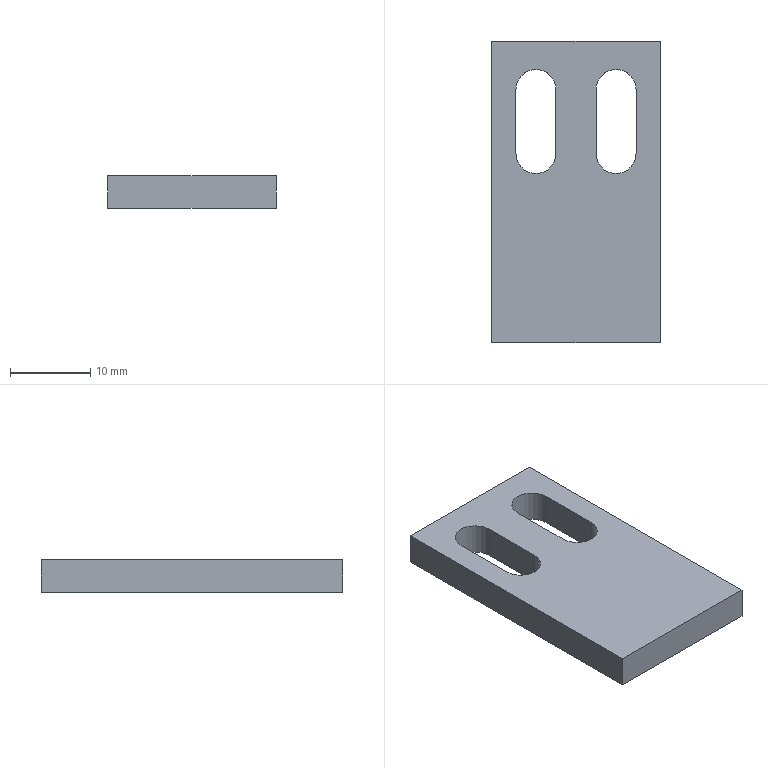Part | STEP file | Sensor spacer block | 1 solid | 14 faces | box 21 x 37.576 x 4 mm | volume 2679 mm3 | plane 10 | cylinder 4 | commonest cylinder face diameters 5 x4
STEP:
#1=CARTESIAN_POINT('',(-11.,-10.,0.));
#2=VERTEX_POINT('',#1);
#3=CARTESIAN_POINT('',(-11.,-47.576,0.));
#4=VERTEX_POINT('',#3);
#5=CARTESIAN_POINT('',(-11.,-10.,0.));
#6=DIRECTION('',(0.,-1.,0.));
#7=VECTOR('',#6,1000.);
#8=LINE('',#5,#7);
#9=EDGE_CURVE('',#2,#4,#8,.T.);
#10=ORIENTED_EDGE('',*,*,#9,.T.);
#11=CARTESIAN_POINT('',(-11.,-47.576,4.));
#12=VERTEX_POINT('',#11);
#13=CARTESIAN_POINT('',(-11.,-47.576,4.));
#14=DIRECTION('',(0.,0.,-1.));
#15=VECTOR('',#14,1000.);
#16=LINE('',#13,#15);
#17=EDGE_CURVE('',#12,#4,#16,.T.);
#18=ORIENTED_EDGE('',*,*,#17,.F.);
#19=CARTESIAN_POINT('',(-11.,-10.,4.));
#20=VERTEX_POINT('',#19);
#21=CARTESIAN_POINT('',(-11.,-10.,4.));
#22=DIRECTION('',(0.,-1.,0.));
#23=VECTOR('',#22,1000.);
#24=LINE('',#21,#23);
#25=EDGE_CURVE('',#20,#12,#24,.T.);
#26=ORIENTED_EDGE('',*,*,#25,.F.);
#27=CARTESIAN_POINT('',(-11.,-10.,4.));
#28=DIRECTION('',(0.,0.,-1.));
#29=VECTOR('',#28,1000.);
#30=LINE('',#27,#29);
#31=EDGE_CURVE('',#20,#2,#30,.T.);
#32=ORIENTED_EDGE('',*,*,#31,.T.);
#33=EDGE_LOOP('',(#10,#18,#26,#32));
#34=FACE_OUTER_BOUND('',#33,.T.);
#35=CARTESIAN_POINT('',(-11.,-10.,4.));
#36=DIRECTION('',(1.,0.,0.));
#37=DIRECTION('',(0.,0.,-1.));
#38=AXIS2_PLACEMENT_3D('',#35,#36,#37);
#39=PLANE('',#38);
#40=ADVANCED_FACE('',(#34),#39,.F.);
#41=CARTESIAN_POINT('',(10.,-47.576,0.));
#42=VERTEX_POINT('',#41);
#43=CARTESIAN_POINT('',(-11.,-47.576,0.));
#44=DIRECTION('',(1.,0.,0.));
#45=VECTOR('',#44,1000.);
#46=LINE('',#43,#45);
#47=EDGE_CURVE('',#4,#42,#46,.T.);
#48=ORIENTED_EDGE('',*,*,#47,.T.);
#49=CARTESIAN_POINT('',(10.,-47.576,4.));
#50=VERTEX_POINT('',#49);
#51=CARTESIAN_POINT('',(10.,-47.576,4.));
#52=DIRECTION('',(0.,0.,-1.));
#53=VECTOR('',#52,1000.);
#54=LINE('',#51,#53);
#55=EDGE_CURVE('',#50,#42,#54,.T.);
#56=ORIENTED_EDGE('',*,*,#55,.F.);
#57=CARTESIAN_POINT('',(-11.,-47.576,4.));
#58=DIRECTION('',(1.,0.,0.));
#59=VECTOR('',#58,1000.);
#60=LINE('',#57,#59);
#61=EDGE_CURVE('',#12,#50,#60,.T.);
#62=ORIENTED_EDGE('',*,*,#61,.F.);
#63=ORIENTED_EDGE('',*,*,#17,.T.);
#64=EDGE_LOOP('',(#48,#56,#62,#63));
#65=FACE_OUTER_BOUND('',#64,.T.);
#66=CARTESIAN_POINT('',(-11.,-47.576,4.));
#67=DIRECTION('',(0.,1.,0.));
#68=DIRECTION('',(0.,0.,1.));
#69=AXIS2_PLACEMENT_3D('',#66,#67,#68);
#70=PLANE('',#69);
#71=ADVANCED_FACE('',(#65),#70,.F.);
#72=CARTESIAN_POINT('',(10.,-10.,0.));
#73=VERTEX_POINT('',#72);
#74=CARTESIAN_POINT('',(10.,-10.,0.));
#75=DIRECTION('',(0.,1.,0.));
#76=VECTOR('',#75,1000.);
#77=LINE('',#74,#76);
#78=EDGE_CURVE('',#42,#73,#77,.T.);
#79=ORIENTED_EDGE('',*,*,#78,.T.);
#80=CARTESIAN_POINT('',(10.,-10.,4.));
#81=VERTEX_POINT('',#80);
#82=CARTESIAN_POINT('',(10.,-10.,4.));
#83=DIRECTION('',(0.,0.,-1.));
#84=VECTOR('',#83,1000.);
#85=LINE('',#82,#84);
#86=EDGE_CURVE('',#81,#73,#85,.T.);
#87=ORIENTED_EDGE('',*,*,#86,.F.);
#88=CARTESIAN_POINT('',(10.,-10.,4.));
#89=DIRECTION('',(0.,1.,0.));
#90=VECTOR('',#89,1000.);
#91=LINE('',#88,#90);
#92=EDGE_CURVE('',#50,#81,#91,.T.);
#93=ORIENTED_EDGE('',*,*,#92,.F.);
#94=ORIENTED_EDGE('',*,*,#55,.T.);
#95=EDGE_LOOP('',(#79,#87,#93,#94));
#96=FACE_OUTER_BOUND('',#95,.T.);
#97=CARTESIAN_POINT('',(10.,-10.,4.));
#98=DIRECTION('',(-1.,0.,0.));
#99=DIRECTION('',(0.,-1.,0.));
#100=AXIS2_PLACEMENT_3D('',#97,#98,#99);
#101=PLANE('',#100);
#102=ADVANCED_FACE('',(#96),#101,.F.);
#103=CARTESIAN_POINT('',(-11.,-10.,0.));
#104=DIRECTION('',(-1.,0.,0.));
#105=VECTOR('',#104,1000.);
#106=LINE('',#103,#105);
#107=EDGE_CURVE('',#73,#2,#106,.T.);
#108=ORIENTED_EDGE('',*,*,#107,.T.);
#109=ORIENTED_EDGE('',*,*,#31,.F.);
#110=CARTESIAN_POINT('',(-11.,-10.,4.));
#111=DIRECTION('',(-1.,0.,0.));
#112=VECTOR('',#111,1000.);
#113=LINE('',#110,#112);
#114=EDGE_CURVE('',#81,#20,#113,.T.);
#115=ORIENTED_EDGE('',*,*,#114,.F.);
#116=ORIENTED_EDGE('',*,*,#86,.T.);
#117=EDGE_LOOP('',(#108,#109,#115,#116));
#118=FACE_OUTER_BOUND('',#117,.T.);
#119=CARTESIAN_POINT('',(-11.,-10.,4.));
#120=DIRECTION('',(0.,-1.,0.));
#121=DIRECTION('',(0.,0.,-1.));
#122=AXIS2_PLACEMENT_3D('',#119,#120,#121);
#123=PLANE('',#122);
#124=ADVANCED_FACE('',(#118),#123,.F.);
#125=CARTESIAN_POINT('',(-3.,-16.,4.));
#126=VERTEX_POINT('',#125);
#127=CARTESIAN_POINT('',(-8.,-16.,4.));
#128=VERTEX_POINT('',#127);
#129=CARTESIAN_POINT('',(-5.5,-16.,4.));
#130=DIRECTION('',(0.,0.,1.));
#131=DIRECTION('',(1.,0.,0.));
#132=AXIS2_PLACEMENT_3D('',#129,#130,#131);
#133=CIRCLE('',#132,2.5);
#134=EDGE_CURVE('',#126,#128,#133,.T.);
#135=ORIENTED_EDGE('',*,*,#134,.F.);
#136=CARTESIAN_POINT('',(-3.,-24.,4.));
#137=VERTEX_POINT('',#136);
#138=CARTESIAN_POINT('',(-3.,-16.,4.));
#139=DIRECTION('',(0.,1.,0.));
#140=VECTOR('',#139,1000.);
#141=LINE('',#138,#140);
#142=EDGE_CURVE('',#137,#126,#141,.T.);
#143=ORIENTED_EDGE('',*,*,#142,.F.);
#144=CARTESIAN_POINT('',(-8.,-24.,4.));
#145=VERTEX_POINT('',#144);
#146=CARTESIAN_POINT('',(-5.5,-24.,4.));
#147=DIRECTION('',(0.,0.,1.));
#148=DIRECTION('',(1.,0.,0.));
#149=AXIS2_PLACEMENT_3D('',#146,#147,#148);
#150=CIRCLE('',#149,2.5);
#151=EDGE_CURVE('',#145,#137,#150,.T.);
#152=ORIENTED_EDGE('',*,*,#151,.F.);
#153=CARTESIAN_POINT('',(-8.,-16.,4.));
#154=DIRECTION('',(0.,-1.,0.));
#155=VECTOR('',#154,1000.);
#156=LINE('',#153,#155);
#157=EDGE_CURVE('',#128,#145,#156,.T.);
#158=ORIENTED_EDGE('',*,*,#157,.F.);
#159=EDGE_LOOP('',(#135,#143,#152,#158));
#160=FACE_BOUND('',#159,.T.);
#161=CARTESIAN_POINT('',(7.,-16.,4.));
#162=VERTEX_POINT('',#161);
#163=CARTESIAN_POINT('',(2.,-16.,4.));
#164=VERTEX_POINT('',#163);
#165=CARTESIAN_POINT('',(4.5,-16.,4.));
#166=DIRECTION('',(0.,0.,1.));
#167=DIRECTION('',(-1.,0.,0.));
#168=AXIS2_PLACEMENT_3D('',#165,#166,#167);
#169=CIRCLE('',#168,2.5);
#170=EDGE_CURVE('',#162,#164,#169,.T.);
#171=ORIENTED_EDGE('',*,*,#170,.F.);
#172=CARTESIAN_POINT('',(7.,-24.,4.));
#173=VERTEX_POINT('',#172);
#174=CARTESIAN_POINT('',(7.,-16.,4.));
#175=DIRECTION('',(0.,1.,0.));
#176=VECTOR('',#175,1000.);
#177=LINE('',#174,#176);
#178=EDGE_CURVE('',#173,#162,#177,.T.);
#179=ORIENTED_EDGE('',*,*,#178,.F.);
#180=CARTESIAN_POINT('',(2.,-24.,4.));
#181=VERTEX_POINT('',#180);
#182=CARTESIAN_POINT('',(4.5,-24.,4.));
#183=DIRECTION('',(0.,0.,1.));
#184=DIRECTION('',(-1.,0.,0.));
#185=AXIS2_PLACEMENT_3D('',#182,#183,#184);
#186=CIRCLE('',#185,2.5);
#187=EDGE_CURVE('',#181,#173,#186,.T.);
#188=ORIENTED_EDGE('',*,*,#187,.F.);
#189=CARTESIAN_POINT('',(2.,-16.,4.));
#190=DIRECTION('',(0.,-1.,0.));
#191=VECTOR('',#190,1000.);
#192=LINE('',#189,#191);
#193=EDGE_CURVE('',#164,#181,#192,.T.);
#194=ORIENTED_EDGE('',*,*,#193,.F.);
#195=EDGE_LOOP('',(#171,#179,#188,#194));
#196=FACE_BOUND('',#195,.T.);
#197=ORIENTED_EDGE('',*,*,#25,.T.);
#198=ORIENTED_EDGE('',*,*,#61,.T.);
#199=ORIENTED_EDGE('',*,*,#92,.T.);
#200=ORIENTED_EDGE('',*,*,#114,.T.);
#201=EDGE_LOOP('',(#197,#198,#199,#200));
#202=FACE_OUTER_BOUND('',#201,.T.);
#203=CARTESIAN_POINT('',(0.,0.,4.));
#204=DIRECTION('',(0.,0.,1.));
#205=DIRECTION('',(1.,0.,0.));
#206=AXIS2_PLACEMENT_3D('',#203,#204,#205);
#207=PLANE('',#206);
#208=ADVANCED_FACE('',(#160,#196,#202),#207,.T.);
#209=CARTESIAN_POINT('',(-3.,-16.,0.));
#210=VERTEX_POINT('',#209);
#211=CARTESIAN_POINT('',(-3.,-24.,0.));
#212=VERTEX_POINT('',#211);
#213=CARTESIAN_POINT('',(-3.,-16.,0.));
#214=DIRECTION('',(0.,-1.,0.));
#215=VECTOR('',#214,1000.);
#216=LINE('',#213,#215);
#217=EDGE_CURVE('',#210,#212,#216,.T.);
#218=ORIENTED_EDGE('',*,*,#217,.F.);
#219=CARTESIAN_POINT('',(-8.,-16.,0.));
#220=VERTEX_POINT('',#219);
#221=CARTESIAN_POINT('',(-5.5,-16.,0.));
#222=DIRECTION('',(0.,0.,-1.));
#223=DIRECTION('',(1.,0.,0.));
#224=AXIS2_PLACEMENT_3D('',#221,#222,#223);
#225=CIRCLE('',#224,2.5);
#226=EDGE_CURVE('',#220,#210,#225,.T.);
#227=ORIENTED_EDGE('',*,*,#226,.F.);
#228=CARTESIAN_POINT('',(-8.,-24.,0.));
#229=VERTEX_POINT('',#228);
#230=CARTESIAN_POINT('',(-8.,-16.,0.));
#231=DIRECTION('',(0.,1.,0.));
#232=VECTOR('',#231,1000.);
#233=LINE('',#230,#232);
#234=EDGE_CURVE('',#229,#220,#233,.T.);
#235=ORIENTED_EDGE('',*,*,#234,.F.);
#236=CARTESIAN_POINT('',(-5.5,-24.,0.));
#237=DIRECTION('',(0.,0.,-1.));
#238=DIRECTION('',(1.,0.,0.));
#239=AXIS2_PLACEMENT_3D('',#236,#237,#238);
#240=CIRCLE('',#239,2.5);
#241=EDGE_CURVE('',#212,#229,#240,.T.);
#242=ORIENTED_EDGE('',*,*,#241,.F.);
#243=EDGE_LOOP('',(#218,#227,#235,#242));
#244=FACE_BOUND('',#243,.T.);
#245=CARTESIAN_POINT('',(7.,-16.,0.));
#246=VERTEX_POINT('',#245);
#247=CARTESIAN_POINT('',(7.,-24.,0.));
#248=VERTEX_POINT('',#247);
#249=CARTESIAN_POINT('',(7.,-16.,0.));
#250=DIRECTION('',(0.,-1.,0.));
#251=VECTOR('',#250,1000.);
#252=LINE('',#249,#251);
#253=EDGE_CURVE('',#246,#248,#252,.T.);
#254=ORIENTED_EDGE('',*,*,#253,.F.);
#255=CARTESIAN_POINT('',(2.,-16.,0.));
#256=VERTEX_POINT('',#255);
#257=CARTESIAN_POINT('',(4.5,-16.,0.));
#258=DIRECTION('',(0.,0.,-1.));
#259=DIRECTION('',(1.,0.,0.));
#260=AXIS2_PLACEMENT_3D('',#257,#258,#259);
#261=CIRCLE('',#260,2.5);
#262=EDGE_CURVE('',#256,#246,#261,.T.);
#263=ORIENTED_EDGE('',*,*,#262,.F.);
#264=CARTESIAN_POINT('',(2.,-24.,0.));
#265=VERTEX_POINT('',#264);
#266=CARTESIAN_POINT('',(2.,-16.,0.));
#267=DIRECTION('',(0.,1.,0.));
#268=VECTOR('',#267,1000.);
#269=LINE('',#266,#268);
#270=EDGE_CURVE('',#265,#256,#269,.T.);
#271=ORIENTED_EDGE('',*,*,#270,.F.);
#272=CARTESIAN_POINT('',(4.5,-24.,0.));
#273=DIRECTION('',(0.,0.,-1.));
#274=DIRECTION('',(1.,0.,0.));
#275=AXIS2_PLACEMENT_3D('',#272,#273,#274);
#276=CIRCLE('',#275,2.5);
#277=EDGE_CURVE('',#248,#265,#276,.T.);
#278=ORIENTED_EDGE('',*,*,#277,.F.);
#279=EDGE_LOOP('',(#254,#263,#271,#278));
#280=FACE_BOUND('',#279,.T.);
#281=ORIENTED_EDGE('',*,*,#9,.F.);
#282=ORIENTED_EDGE('',*,*,#107,.F.);
#283=ORIENTED_EDGE('',*,*,#78,.F.);
#284=ORIENTED_EDGE('',*,*,#47,.F.);
#285=EDGE_LOOP('',(#281,#282,#283,#284));
#286=FACE_OUTER_BOUND('',#285,.T.);
#287=CARTESIAN_POINT('',(0.,0.,0.));
#288=DIRECTION('',(0.,0.,1.));
#289=DIRECTION('',(1.,0.,0.));
#290=AXIS2_PLACEMENT_3D('',#287,#288,#289);
#291=PLANE('',#290);
#292=ADVANCED_FACE('',(#244,#280,#286),#291,.F.);
#293=ORIENTED_EDGE('',*,*,#262,.T.);
#294=CARTESIAN_POINT('',(7.,-16.,-0.001));
#295=DIRECTION('',(0.,0.,1.));
#296=VECTOR('',#295,1000.);
#297=LINE('',#294,#296);
#298=EDGE_CURVE('',#246,#162,#297,.T.);
#299=ORIENTED_EDGE('',*,*,#298,.T.);
#300=ORIENTED_EDGE('',*,*,#170,.T.);
#301=CARTESIAN_POINT('',(2.,-16.,-0.001));
#302=DIRECTION('',(0.,0.,1.));
#303=VECTOR('',#302,1000.);
#304=LINE('',#301,#303);
#305=EDGE_CURVE('',#256,#164,#304,.T.);
#306=ORIENTED_EDGE('',*,*,#305,.F.);
#307=EDGE_LOOP('',(#293,#299,#300,#306));
#308=FACE_OUTER_BOUND('',#307,.T.);
#309=CARTESIAN_POINT('',(4.5,-16.,-0.001));
#310=DIRECTION('',(0.,0.,1.));
#311=DIRECTION('',(1.,0.,0.));
#312=AXIS2_PLACEMENT_3D('',#309,#310,#311);
#313=CYLINDRICAL_SURFACE('',#312,2.5);
#314=ADVANCED_FACE('',(#308),#313,.F.);
#315=ORIENTED_EDGE('',*,*,#253,.T.);
#316=CARTESIAN_POINT('',(7.,-24.,-0.001));
#317=DIRECTION('',(0.,0.,1.));
#318=VECTOR('',#317,1000.);
#319=LINE('',#316,#318);
#320=EDGE_CURVE('',#248,#173,#319,.T.);
#321=ORIENTED_EDGE('',*,*,#320,.T.);
#322=ORIENTED_EDGE('',*,*,#178,.T.);
#323=ORIENTED_EDGE('',*,*,#298,.F.);
#324=EDGE_LOOP('',(#315,#321,#322,#323));
#325=FACE_OUTER_BOUND('',#324,.T.);
#326=CARTESIAN_POINT('',(7.,-16.,-0.001));
#327=DIRECTION('',(1.,0.,0.));
#328=DIRECTION('',(0.,1.,0.));
#329=AXIS2_PLACEMENT_3D('',#326,#327,#328);
#330=PLANE('',#329);
#331=ADVANCED_FACE('',(#325),#330,.F.);
#332=ORIENTED_EDGE('',*,*,#277,.T.);
#333=CARTESIAN_POINT('',(2.,-24.,-0.001));
#334=DIRECTION('',(0.,0.,1.));
#335=VECTOR('',#334,1000.);
#336=LINE('',#333,#335);
#337=EDGE_CURVE('',#265,#181,#336,.T.);
#338=ORIENTED_EDGE('',*,*,#337,.T.);
#339=ORIENTED_EDGE('',*,*,#187,.T.);
#340=ORIENTED_EDGE('',*,*,#320,.F.);
#341=EDGE_LOOP('',(#332,#338,#339,#340));
#342=FACE_OUTER_BOUND('',#341,.T.);
#343=CARTESIAN_POINT('',(4.5,-24.,-0.001));
#344=DIRECTION('',(0.,0.,1.));
#345=DIRECTION('',(1.,0.,0.));
#346=AXIS2_PLACEMENT_3D('',#343,#344,#345);
#347=CYLINDRICAL_SURFACE('',#346,2.5);
#348=ADVANCED_FACE('',(#342),#347,.F.);
#349=ORIENTED_EDGE('',*,*,#270,.T.);
#350=ORIENTED_EDGE('',*,*,#305,.T.);
#351=ORIENTED_EDGE('',*,*,#193,.T.);
#352=ORIENTED_EDGE('',*,*,#337,.F.);
#353=EDGE_LOOP('',(#349,#350,#351,#352));
#354=FACE_OUTER_BOUND('',#353,.T.);
#355=CARTESIAN_POINT('',(2.,-16.,-0.001));
#356=DIRECTION('',(-1.,0.,0.));
#357=DIRECTION('',(0.,-1.,0.));
#358=AXIS2_PLACEMENT_3D('',#355,#356,#357);
#359=PLANE('',#358);
#360=ADVANCED_FACE('',(#354),#359,.F.);
#361=ORIENTED_EDGE('',*,*,#226,.T.);
#362=CARTESIAN_POINT('',(-3.,-16.,-0.001));
#363=DIRECTION('',(0.,0.,1.));
#364=VECTOR('',#363,1000.);
#365=LINE('',#362,#364);
#366=EDGE_CURVE('',#210,#126,#365,.T.);
#367=ORIENTED_EDGE('',*,*,#366,.T.);
#368=ORIENTED_EDGE('',*,*,#134,.T.);
#369=CARTESIAN_POINT('',(-8.,-16.,-0.001));
#370=DIRECTION('',(0.,0.,1.));
#371=VECTOR('',#370,1000.);
#372=LINE('',#369,#371);
#373=EDGE_CURVE('',#220,#128,#372,.T.);
#374=ORIENTED_EDGE('',*,*,#373,.F.);
#375=EDGE_LOOP('',(#361,#367,#368,#374));
#376=FACE_OUTER_BOUND('',#375,.T.);
#377=CARTESIAN_POINT('',(-5.5,-16.,-0.001));
#378=DIRECTION('',(0.,0.,1.));
#379=DIRECTION('',(1.,0.,0.));
#380=AXIS2_PLACEMENT_3D('',#377,#378,#379);
#381=CYLINDRICAL_SURFACE('',#380,2.5);
#382=ADVANCED_FACE('',(#376),#381,.F.);
#383=ORIENTED_EDGE('',*,*,#217,.T.);
#384=CARTESIAN_POINT('',(-3.,-24.,-0.001));
#385=DIRECTION('',(0.,0.,1.));
#386=VECTOR('',#385,1000.);
#387=LINE('',#384,#386);
#388=EDGE_CURVE('',#212,#137,#387,.T.);
#389=ORIENTED_EDGE('',*,*,#388,.T.);
#390=ORIENTED_EDGE('',*,*,#142,.T.);
#391=ORIENTED_EDGE('',*,*,#366,.F.);
#392=EDGE_LOOP('',(#383,#389,#390,#391));
#393=FACE_OUTER_BOUND('',#392,.T.);
#394=CARTESIAN_POINT('',(-3.,-16.,-0.001));
#395=DIRECTION('',(1.,0.,0.));
#396=DIRECTION('',(0.,1.,0.));
#397=AXIS2_PLACEMENT_3D('',#394,#395,#396);
#398=PLANE('',#397);
#399=ADVANCED_FACE('',(#393),#398,.F.);
#400=ORIENTED_EDGE('',*,*,#241,.T.);
#401=CARTESIAN_POINT('',(-8.,-24.,-0.001));
#402=DIRECTION('',(0.,0.,1.));
#403=VECTOR('',#402,1000.);
#404=LINE('',#401,#403);
#405=EDGE_CURVE('',#229,#145,#404,.T.);
#406=ORIENTED_EDGE('',*,*,#405,.T.);
#407=ORIENTED_EDGE('',*,*,#151,.T.);
#408=ORIENTED_EDGE('',*,*,#388,.F.);
#409=EDGE_LOOP('',(#400,#406,#407,#408));
#410=FACE_OUTER_BOUND('',#409,.T.);
#411=CARTESIAN_POINT('',(-5.5,-24.,-0.001));
#412=DIRECTION('',(0.,0.,1.));
#413=DIRECTION('',(1.,0.,0.));
#414=AXIS2_PLACEMENT_3D('',#411,#412,#413);
#415=CYLINDRICAL_SURFACE('',#414,2.5);
#416=ADVANCED_FACE('',(#410),#415,.F.);
#417=ORIENTED_EDGE('',*,*,#234,.T.);
#418=ORIENTED_EDGE('',*,*,#373,.T.);
#419=ORIENTED_EDGE('',*,*,#157,.T.);
#420=ORIENTED_EDGE('',*,*,#405,.F.);
#421=EDGE_LOOP('',(#417,#418,#419,#420));
#422=FACE_OUTER_BOUND('',#421,.T.);
#423=CARTESIAN_POINT('',(-8.,-16.,-0.001));
#424=DIRECTION('',(-1.,0.,0.));
#425=DIRECTION('',(0.,-1.,0.));
#426=AXIS2_PLACEMENT_3D('',#423,#424,#425);
#427=PLANE('',#426);
#428=ADVANCED_FACE('',(#422),#427,.F.);
#429=CLOSED_SHELL('',(#40,#71,#102,#124,#208,#292,#314,#331,#348,#360,#382,#399,#416,#428));
#430=MANIFOLD_SOLID_BREP('',#429);
#431=CARTESIAN_POINT('',(0.,0.,0.));
#432=DIRECTION('',(0.,0.,1.));
#433=DIRECTION('',(1.,0.,0.));
#434=AXIS2_PLACEMENT_3D('',#431,#432,#433);
#435=(LENGTH_UNIT()NAMED_UNIT(*)SI_UNIT(.MILLI.,.METRE.));
#436=UNCERTAINTY_MEASURE_WITH_UNIT(LENGTH_MEASURE(0.00001),#435,'','');
#437=(NAMED_UNIT(*)PLANE_ANGLE_UNIT()SI_UNIT($,.RADIAN.));
#438=(NAMED_UNIT(*)SI_UNIT($,.STERADIAN.)SOLID_ANGLE_UNIT());
#439=(GEOMETRIC_REPRESENTATION_CONTEXT(3)GLOBAL_UNCERTAINTY_ASSIGNED_CONTEXT((#436))GLOBAL_UNIT_ASSIGNED_CONTEXT((#435,#437,#438))REPRESENTATION_CONTEXT('',''));
#440=ADVANCED_BREP_SHAPE_REPRESENTATION('',(#430,#434),#439);